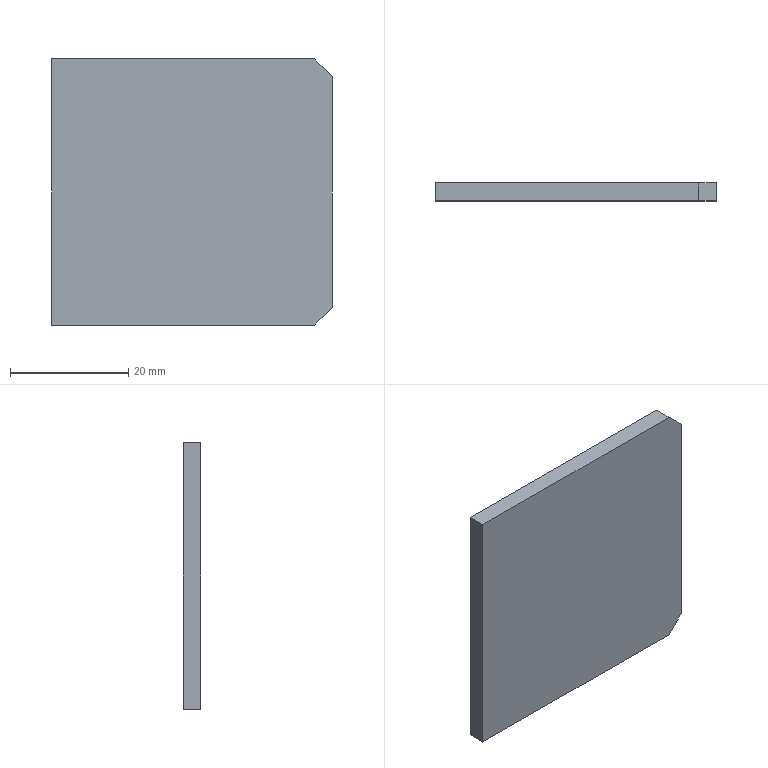Part | SolidWorks | features BaseBody 1 | 1 solid | 8 faces | box 47.5 x 3 x 45 mm | volume 6385 mm3 | plane 8
STEP:
#1=CARTESIAN_POINT('',(944.446,-3645.977,2109.471));
#2=VERTEX_POINT('',#1);
#3=CARTESIAN_POINT('',(944.446,-3645.977,2070.471));
#4=VERTEX_POINT('',#3);
#5=CARTESIAN_POINT('',(944.446,-3645.977,2089.971));
#6=DIRECTION('',(0.,0.,-1.));
#7=VECTOR('',#6,1000.);
#8=LINE('',#5,#7);
#9=EDGE_CURVE('',#2,#4,#8,.T.);
#10=ORIENTED_EDGE('',*,*,#9,.F.);
#11=CARTESIAN_POINT('',(941.446,-3645.977,2112.471));
#12=VERTEX_POINT('',#11);
#13=CARTESIAN_POINT('',(941.446,-3645.977,2112.471));
#14=DIRECTION('',(0.7071,0.,-0.7071));
#15=VECTOR('',#14,1000.);
#16=LINE('',#13,#15);
#17=EDGE_CURVE('',#12,#2,#16,.T.);
#18=ORIENTED_EDGE('',*,*,#17,.F.);
#19=CARTESIAN_POINT('',(896.946,-3645.977,2112.471));
#20=VERTEX_POINT('',#19);
#21=CARTESIAN_POINT('',(920.215,-3645.977,2112.471));
#22=DIRECTION('',(1.,0.,0.));
#23=VECTOR('',#22,1000.);
#24=LINE('',#21,#23);
#25=EDGE_CURVE('',#20,#12,#24,.T.);
#26=ORIENTED_EDGE('',*,*,#25,.F.);
#27=CARTESIAN_POINT('',(896.946,-3645.977,2067.471));
#28=VERTEX_POINT('',#27);
#29=CARTESIAN_POINT('',(896.946,-3645.977,2089.971));
#30=DIRECTION('',(0.,0.,1.));
#31=VECTOR('',#30,1000.);
#32=LINE('',#29,#31);
#33=EDGE_CURVE('',#28,#20,#32,.T.);
#34=ORIENTED_EDGE('',*,*,#33,.F.);
#35=CARTESIAN_POINT('',(941.446,-3645.977,2067.471));
#36=VERTEX_POINT('',#35);
#37=CARTESIAN_POINT('',(920.215,-3645.977,2067.471));
#38=DIRECTION('',(-1.,0.,0.));
#39=VECTOR('',#38,1000.);
#40=LINE('',#37,#39);
#41=EDGE_CURVE('',#36,#28,#40,.T.);
#42=ORIENTED_EDGE('',*,*,#41,.F.);
#43=CARTESIAN_POINT('',(944.446,-3645.977,2070.471));
#44=DIRECTION('',(-0.7071,0.,-0.7071));
#45=VECTOR('',#44,1000.);
#46=LINE('',#43,#45);
#47=EDGE_CURVE('',#4,#36,#46,.T.);
#48=ORIENTED_EDGE('',*,*,#47,.F.);
#49=EDGE_LOOP('',(#10,#18,#26,#34,#42,#48));
#50=FACE_OUTER_BOUND('',#49,.T.);
#51=CARTESIAN_POINT('',(920.215,-3645.977,2089.971));
#52=DIRECTION('',(0.,1.,0.));
#53=DIRECTION('',(0.,0.,1.));
#54=AXIS2_PLACEMENT_3D('',#51,#52,#53);
#55=PLANE('',#54);
#56=ADVANCED_FACE('',(#50),#55,.F.);
#57=CARTESIAN_POINT('',(941.446,-3642.977,2067.471));
#58=VERTEX_POINT('',#57);
#59=CARTESIAN_POINT('',(944.446,-3642.977,2070.471));
#60=VERTEX_POINT('',#59);
#61=CARTESIAN_POINT('',(941.446,-3642.977,2067.471));
#62=DIRECTION('',(0.7071,0.,0.7071));
#63=VECTOR('',#62,1000.);
#64=LINE('',#61,#63);
#65=EDGE_CURVE('',#58,#60,#64,.T.);
#66=ORIENTED_EDGE('',*,*,#65,.T.);
#67=CARTESIAN_POINT('',(944.446,-3642.977,2070.471));
#68=DIRECTION('',(0.,-1.,0.));
#69=VECTOR('',#68,1000.);
#70=LINE('',#67,#69);
#71=EDGE_CURVE('',#60,#4,#70,.T.);
#72=ORIENTED_EDGE('',*,*,#71,.T.);
#73=ORIENTED_EDGE('',*,*,#47,.T.);
#74=CARTESIAN_POINT('',(941.446,-3642.977,2067.471));
#75=DIRECTION('',(0.,1.,0.));
#76=VECTOR('',#75,1000.);
#77=LINE('',#74,#76);
#78=EDGE_CURVE('',#36,#58,#77,.T.);
#79=ORIENTED_EDGE('',*,*,#78,.T.);
#80=EDGE_LOOP('',(#66,#72,#73,#79));
#81=FACE_OUTER_BOUND('',#80,.T.);
#82=CARTESIAN_POINT('',(941.446,-3642.977,2067.471));
#83=DIRECTION('',(0.7071,0.,-0.7071));
#84=DIRECTION('',(-0.7071,0.,-0.7071));
#85=AXIS2_PLACEMENT_3D('',#82,#83,#84);
#86=PLANE('',#85);
#87=ADVANCED_FACE('',(#81),#86,.T.);
#88=CARTESIAN_POINT('',(944.446,-3642.977,2109.471));
#89=VERTEX_POINT('',#88);
#90=CARTESIAN_POINT('',(944.446,-3642.977,2070.471));
#91=DIRECTION('',(0.,0.,1.));
#92=VECTOR('',#91,1000.);
#93=LINE('',#90,#92);
#94=EDGE_CURVE('',#60,#89,#93,.T.);
#95=ORIENTED_EDGE('',*,*,#94,.T.);
#96=CARTESIAN_POINT('',(944.446,-3642.977,2109.471));
#97=DIRECTION('',(0.,-1.,0.));
#98=VECTOR('',#97,1000.);
#99=LINE('',#96,#98);
#100=EDGE_CURVE('',#89,#2,#99,.T.);
#101=ORIENTED_EDGE('',*,*,#100,.T.);
#102=ORIENTED_EDGE('',*,*,#9,.T.);
#103=ORIENTED_EDGE('',*,*,#71,.F.);
#104=EDGE_LOOP('',(#95,#101,#102,#103));
#105=FACE_OUTER_BOUND('',#104,.T.);
#106=CARTESIAN_POINT('',(944.446,-3642.977,2070.471));
#107=DIRECTION('',(1.,0.,0.));
#108=DIRECTION('',(0.,0.,-1.));
#109=AXIS2_PLACEMENT_3D('',#106,#107,#108);
#110=PLANE('',#109);
#111=ADVANCED_FACE('',(#105),#110,.T.);
#112=CARTESIAN_POINT('',(941.446,-3642.977,2112.471));
#113=VERTEX_POINT('',#112);
#114=CARTESIAN_POINT('',(944.446,-3642.977,2109.471));
#115=DIRECTION('',(-0.7071,0.,0.7071));
#116=VECTOR('',#115,1000.);
#117=LINE('',#114,#116);
#118=EDGE_CURVE('',#89,#113,#117,.T.);
#119=ORIENTED_EDGE('',*,*,#118,.T.);
#120=CARTESIAN_POINT('',(941.446,-3642.977,2112.471));
#121=DIRECTION('',(0.,-1.,0.));
#122=VECTOR('',#121,1000.);
#123=LINE('',#120,#122);
#124=EDGE_CURVE('',#113,#12,#123,.T.);
#125=ORIENTED_EDGE('',*,*,#124,.T.);
#126=ORIENTED_EDGE('',*,*,#17,.T.);
#127=ORIENTED_EDGE('',*,*,#100,.F.);
#128=EDGE_LOOP('',(#119,#125,#126,#127));
#129=FACE_OUTER_BOUND('',#128,.T.);
#130=CARTESIAN_POINT('',(944.446,-3642.977,2109.471));
#131=DIRECTION('',(0.7071,0.,0.7071));
#132=DIRECTION('',(0.7071,0.,-0.7071));
#133=AXIS2_PLACEMENT_3D('',#130,#131,#132);
#134=PLANE('',#133);
#135=ADVANCED_FACE('',(#129),#134,.T.);
#136=CARTESIAN_POINT('',(896.946,-3642.977,2112.471));
#137=VERTEX_POINT('',#136);
#138=CARTESIAN_POINT('',(941.446,-3642.977,2112.471));
#139=DIRECTION('',(-1.,0.,0.));
#140=VECTOR('',#139,1000.);
#141=LINE('',#138,#140);
#142=EDGE_CURVE('',#113,#137,#141,.T.);
#143=ORIENTED_EDGE('',*,*,#142,.T.);
#144=CARTESIAN_POINT('',(896.946,-3642.977,2112.471));
#145=DIRECTION('',(0.,-1.,0.));
#146=VECTOR('',#145,1000.);
#147=LINE('',#144,#146);
#148=EDGE_CURVE('',#137,#20,#147,.T.);
#149=ORIENTED_EDGE('',*,*,#148,.T.);
#150=ORIENTED_EDGE('',*,*,#25,.T.);
#151=ORIENTED_EDGE('',*,*,#124,.F.);
#152=EDGE_LOOP('',(#143,#149,#150,#151));
#153=FACE_OUTER_BOUND('',#152,.T.);
#154=CARTESIAN_POINT('',(941.446,-3642.977,2112.471));
#155=DIRECTION('',(0.,0.,1.));
#156=DIRECTION('',(1.,0.,0.));
#157=AXIS2_PLACEMENT_3D('',#154,#155,#156);
#158=PLANE('',#157);
#159=ADVANCED_FACE('',(#153),#158,.T.);
#160=CARTESIAN_POINT('',(896.946,-3642.977,2067.471));
#161=VERTEX_POINT('',#160);
#162=CARTESIAN_POINT('',(896.946,-3642.977,2112.471));
#163=DIRECTION('',(0.,0.,-1.));
#164=VECTOR('',#163,1000.);
#165=LINE('',#162,#164);
#166=EDGE_CURVE('',#137,#161,#165,.T.);
#167=ORIENTED_EDGE('',*,*,#166,.T.);
#168=CARTESIAN_POINT('',(896.946,-3642.977,2067.471));
#169=DIRECTION('',(0.,-1.,0.));
#170=VECTOR('',#169,1000.);
#171=LINE('',#168,#170);
#172=EDGE_CURVE('',#161,#28,#171,.T.);
#173=ORIENTED_EDGE('',*,*,#172,.T.);
#174=ORIENTED_EDGE('',*,*,#33,.T.);
#175=ORIENTED_EDGE('',*,*,#148,.F.);
#176=EDGE_LOOP('',(#167,#173,#174,#175));
#177=FACE_OUTER_BOUND('',#176,.T.);
#178=CARTESIAN_POINT('',(896.946,-3642.977,2112.471));
#179=DIRECTION('',(-1.,0.,0.));
#180=DIRECTION('',(0.,0.,1.));
#181=AXIS2_PLACEMENT_3D('',#178,#179,#180);
#182=PLANE('',#181);
#183=ADVANCED_FACE('',(#177),#182,.T.);
#184=CARTESIAN_POINT('',(896.946,-3642.977,2067.471));
#185=DIRECTION('',(1.,0.,0.));
#186=VECTOR('',#185,1000.);
#187=LINE('',#184,#186);
#188=EDGE_CURVE('',#161,#58,#187,.T.);
#189=ORIENTED_EDGE('',*,*,#188,.T.);
#190=ORIENTED_EDGE('',*,*,#78,.F.);
#191=ORIENTED_EDGE('',*,*,#41,.T.);
#192=ORIENTED_EDGE('',*,*,#172,.F.);
#193=EDGE_LOOP('',(#189,#190,#191,#192));
#194=FACE_OUTER_BOUND('',#193,.T.);
#195=CARTESIAN_POINT('',(896.946,-3642.977,2067.471));
#196=DIRECTION('',(0.,0.,-1.));
#197=DIRECTION('',(-1.,0.,0.));
#198=AXIS2_PLACEMENT_3D('',#195,#196,#197);
#199=PLANE('',#198);
#200=ADVANCED_FACE('',(#194),#199,.T.);
#201=ORIENTED_EDGE('',*,*,#94,.F.);
#202=ORIENTED_EDGE('',*,*,#65,.F.);
#203=ORIENTED_EDGE('',*,*,#188,.F.);
#204=ORIENTED_EDGE('',*,*,#166,.F.);
#205=ORIENTED_EDGE('',*,*,#142,.F.);
#206=ORIENTED_EDGE('',*,*,#118,.F.);
#207=EDGE_LOOP('',(#201,#202,#203,#204,#205,#206));
#208=FACE_OUTER_BOUND('',#207,.T.);
#209=CARTESIAN_POINT('',(920.215,-3642.977,2089.971));
#210=DIRECTION('',(0.,1.,0.));
#211=DIRECTION('',(0.,0.,1.));
#212=AXIS2_PLACEMENT_3D('',#209,#210,#211);
#213=PLANE('',#212);
#214=ADVANCED_FACE('',(#208),#213,.T.);
#215=CLOSED_SHELL('',(#56,#87,#111,#135,#159,#183,#200,#214));
#216=MANIFOLD_SOLID_BREP('',#215);
#217=CARTESIAN_POINT('',(0.,0.,0.));
#218=DIRECTION('',(0.,0.,1.));
#219=DIRECTION('',(1.,0.,0.));
#220=AXIS2_PLACEMENT_3D('',#217,#218,#219);
#221=(LENGTH_UNIT()NAMED_UNIT(*)SI_UNIT(.MILLI.,.METRE.));
#222=UNCERTAINTY_MEASURE_WITH_UNIT(LENGTH_MEASURE(0.00001),#221,'','');
#223=(NAMED_UNIT(*)PLANE_ANGLE_UNIT()SI_UNIT($,.RADIAN.));
#224=(NAMED_UNIT(*)SI_UNIT($,.STERADIAN.)SOLID_ANGLE_UNIT());
#225=(GEOMETRIC_REPRESENTATION_CONTEXT(3)GLOBAL_UNCERTAINTY_ASSIGNED_CONTEXT((#222))GLOBAL_UNIT_ASSIGNED_CONTEXT((#221,#223,#224))REPRESENTATION_CONTEXT('',''));
#226=ADVANCED_BREP_SHAPE_REPRESENTATION('',(#216,#220),#225);